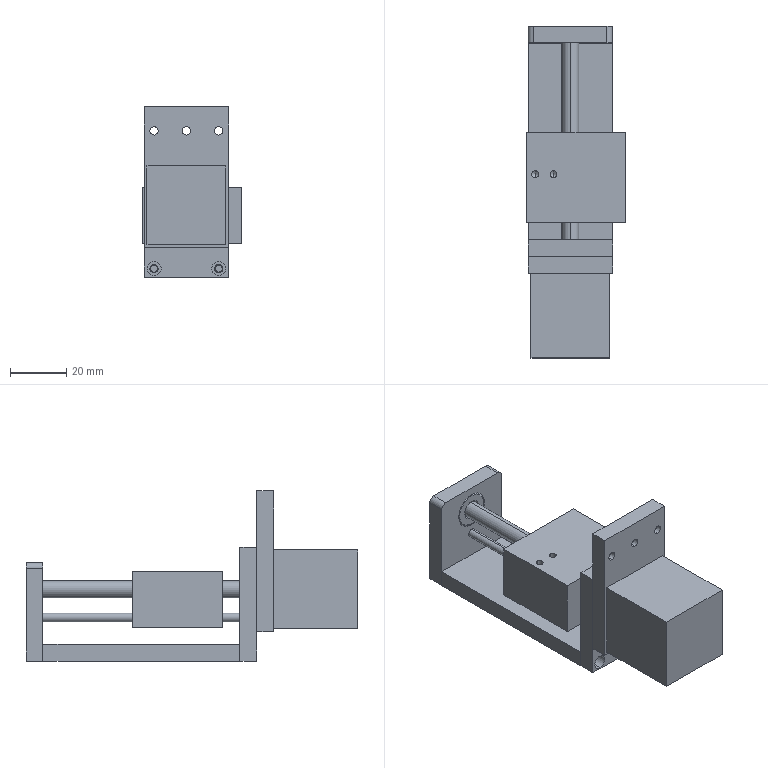Part | SolidWorks | 8 solids | 197 faces | box 35 x 118 x 60.5 mm | volume 80289 mm3 | cylinder 110 | plane 59 | cone 28 | commonest cylinder face diameters 3 x38 2.5 x28 5 x22 6 x8 13 x4 4 x2